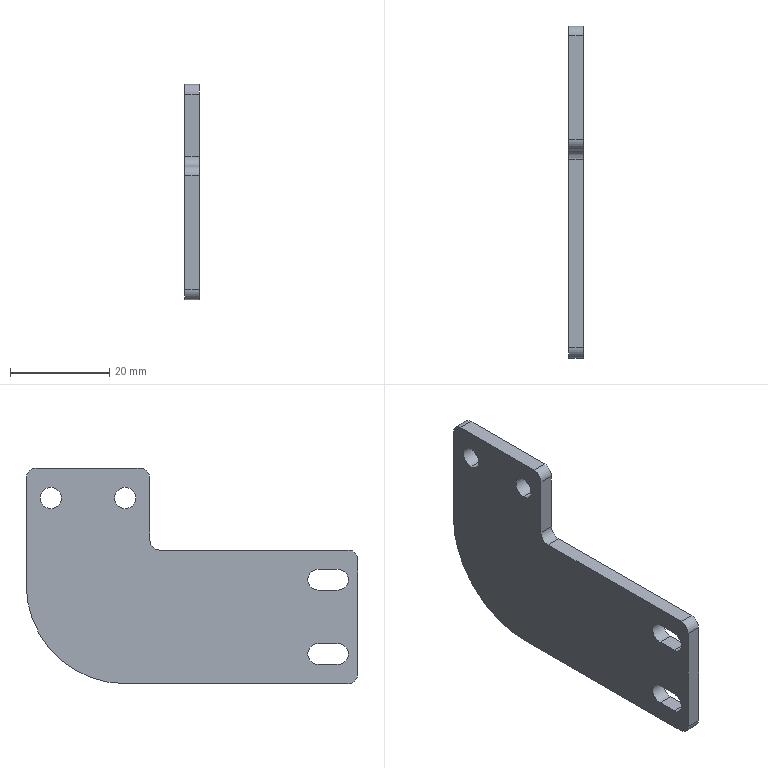Part | SolidWorks | features ICE 5, Fillet 4, Extrusion 1, HoleWzd 1, LPattern 1 | 1 solid | 26 faces | box 3 x 67 x 43.5 mm | volume 6128 mm3 | cylinder 14 | plane 12 | commonest cylinder face diameters 4 x5 4.2 x4 4.3 x4 40 x1
STEP:
#1=CARTESIAN_POINT('',(3.,56.,2.15));
#2=VERTEX_POINT('',#1);
#3=CARTESIAN_POINT('',(3.,56.,-2.15));
#4=VERTEX_POINT('',#3);
#5=CARTESIAN_POINT('',(3.,56.,0.));
#6=DIRECTION('',(1.,0.,0.));
#7=DIRECTION('',(0.,0.,-1.));
#8=AXIS2_PLACEMENT_3D('',#5,#6,#7);
#9=CIRCLE('',#8,2.15);
#10=EDGE_CURVE('',#2,#4,#9,.T.);
#11=ORIENTED_EDGE('',*,*,#10,.T.);
#12=CARTESIAN_POINT('',(0.,56.,-2.15));
#13=VERTEX_POINT('',#12);
#14=CARTESIAN_POINT('',(0.,56.,-2.15));
#15=DIRECTION('',(-1.,0.,0.));
#16=VECTOR('',#15,1000.);
#17=LINE('',#14,#16);
#18=EDGE_CURVE('',#4,#13,#17,.T.);
#19=ORIENTED_EDGE('',*,*,#18,.T.);
#20=CARTESIAN_POINT('',(0.,56.,2.15));
#21=VERTEX_POINT('',#20);
#22=CARTESIAN_POINT('',(0.,56.,0.));
#23=DIRECTION('',(-1.,0.,0.));
#24=DIRECTION('',(0.,0.,1.));
#25=AXIS2_PLACEMENT_3D('',#22,#23,#24);
#26=CIRCLE('',#25,2.15);
#27=EDGE_CURVE('',#13,#21,#26,.T.);
#28=ORIENTED_EDGE('',*,*,#27,.T.);
#29=CARTESIAN_POINT('',(0.,56.,2.15));
#30=DIRECTION('',(-1.,0.,0.));
#31=VECTOR('',#30,1000.);
#32=LINE('',#29,#31);
#33=EDGE_CURVE('',#2,#21,#32,.T.);
#34=ORIENTED_EDGE('',*,*,#33,.F.);
#35=EDGE_LOOP('',(#11,#19,#28,#34));
#36=FACE_OUTER_BOUND('',#35,.T.);
#37=CARTESIAN_POINT('',(0.,56.,0.));
#38=DIRECTION('',(-1.,0.,0.));
#39=DIRECTION('',(0.,0.,1.));
#40=AXIS2_PLACEMENT_3D('',#37,#38,#39);
#41=CYLINDRICAL_SURFACE('',#40,2.15);
#42=ADVANCED_FACE('',(#36),#41,.F.);
#43=CARTESIAN_POINT('',(3.,41.,2.15));
#44=VERTEX_POINT('',#43);
#45=CARTESIAN_POINT('',(3.,41.,-2.15));
#46=VERTEX_POINT('',#45);
#47=CARTESIAN_POINT('',(3.,41.,0.));
#48=DIRECTION('',(1.,0.,0.));
#49=DIRECTION('',(0.,0.,-1.));
#50=AXIS2_PLACEMENT_3D('',#47,#48,#49);
#51=CIRCLE('',#50,2.15);
#52=EDGE_CURVE('',#44,#46,#51,.T.);
#53=ORIENTED_EDGE('',*,*,#52,.T.);
#54=CARTESIAN_POINT('',(0.,41.,-2.15));
#55=VERTEX_POINT('',#54);
#56=CARTESIAN_POINT('',(0.,41.,-2.15));
#57=DIRECTION('',(-1.,0.,0.));
#58=VECTOR('',#57,1000.);
#59=LINE('',#56,#58);
#60=EDGE_CURVE('',#46,#55,#59,.T.);
#61=ORIENTED_EDGE('',*,*,#60,.T.);
#62=CARTESIAN_POINT('',(0.,41.,2.15));
#63=VERTEX_POINT('',#62);
#64=CARTESIAN_POINT('',(0.,41.,0.));
#65=DIRECTION('',(-1.,0.,0.));
#66=DIRECTION('',(0.,0.,1.));
#67=AXIS2_PLACEMENT_3D('',#64,#65,#66);
#68=CIRCLE('',#67,2.15);
#69=EDGE_CURVE('',#55,#63,#68,.T.);
#70=ORIENTED_EDGE('',*,*,#69,.T.);
#71=CARTESIAN_POINT('',(0.,41.,2.15));
#72=DIRECTION('',(-1.,0.,0.));
#73=VECTOR('',#72,1000.);
#74=LINE('',#71,#73);
#75=EDGE_CURVE('',#44,#63,#74,.T.);
#76=ORIENTED_EDGE('',*,*,#75,.F.);
#77=EDGE_LOOP('',(#53,#61,#70,#76));
#78=FACE_OUTER_BOUND('',#77,.T.);
#79=CARTESIAN_POINT('',(0.,41.,0.));
#80=DIRECTION('',(-1.,0.,0.));
#81=DIRECTION('',(0.,0.,1.));
#82=AXIS2_PLACEMENT_3D('',#79,#80,#81);
#83=CYLINDRICAL_SURFACE('',#82,2.15);
#84=ADVANCED_FACE('',(#78),#83,.F.);
#85=CARTESIAN_POINT('',(3.,61.,-17.5));
#86=VERTEX_POINT('',#85);
#87=CARTESIAN_POINT('',(3.,61.,4.));
#88=VERTEX_POINT('',#87);
#89=CARTESIAN_POINT('',(3.,61.,6.));
#90=DIRECTION('',(0.,0.,1.));
#91=VECTOR('',#90,1000.);
#92=LINE('',#89,#91);
#93=EDGE_CURVE('',#86,#88,#92,.T.);
#94=ORIENTED_EDGE('',*,*,#93,.F.);
#95=CARTESIAN_POINT('',(0.,61.,-17.5));
#96=VERTEX_POINT('',#95);
#97=CARTESIAN_POINT('',(0.,61.,-17.5));
#98=DIRECTION('',(-1.,0.,0.));
#99=VECTOR('',#98,1000.);
#100=LINE('',#97,#99);
#101=EDGE_CURVE('',#86,#96,#100,.T.);
#102=ORIENTED_EDGE('',*,*,#101,.T.);
#103=CARTESIAN_POINT('',(0.,61.,4.));
#104=VERTEX_POINT('',#103);
#105=CARTESIAN_POINT('',(0.,61.,6.));
#106=DIRECTION('',(0.,0.,1.));
#107=VECTOR('',#106,1000.);
#108=LINE('',#105,#107);
#109=EDGE_CURVE('',#96,#104,#108,.T.);
#110=ORIENTED_EDGE('',*,*,#109,.T.);
#111=CARTESIAN_POINT('',(3.,61.,4.));
#112=DIRECTION('',(1.,0.,0.));
#113=VECTOR('',#112,1000.);
#114=LINE('',#111,#113);
#115=EDGE_CURVE('',#104,#88,#114,.T.);
#116=ORIENTED_EDGE('',*,*,#115,.T.);
#117=EDGE_LOOP('',(#94,#102,#110,#116));
#118=FACE_OUTER_BOUND('',#117,.T.);
#119=CARTESIAN_POINT('',(3.,61.,6.));
#120=DIRECTION('',(0.,-1.,0.));
#121=DIRECTION('',(0.,0.,-1.));
#122=AXIS2_PLACEMENT_3D('',#119,#120,#121);
#123=PLANE('',#122);
#124=ADVANCED_FACE('',(#118),#123,.F.);
#125=CARTESIAN_POINT('',(3.,-6.,-12.5));
#126=VERTEX_POINT('',#125);
#127=CARTESIAN_POINT('',(3.,-6.,-35.5));
#128=VERTEX_POINT('',#127);
#129=CARTESIAN_POINT('',(3.,-6.,12.5));
#130=DIRECTION('',(0.,0.,-1.));
#131=VECTOR('',#130,1000.);
#132=LINE('',#129,#131);
#133=EDGE_CURVE('',#126,#128,#132,.T.);
#134=ORIENTED_EDGE('',*,*,#133,.F.);
#135=CARTESIAN_POINT('',(0.,-6.,-12.5));
#136=VERTEX_POINT('',#135);
#137=CARTESIAN_POINT('',(0.,-6.,-12.5));
#138=DIRECTION('',(-1.,0.,0.));
#139=VECTOR('',#138,1000.);
#140=LINE('',#137,#139);
#141=EDGE_CURVE('',#126,#136,#140,.T.);
#142=ORIENTED_EDGE('',*,*,#141,.T.);
#143=CARTESIAN_POINT('',(0.,-6.,-35.5));
#144=VERTEX_POINT('',#143);
#145=CARTESIAN_POINT('',(0.,-6.,12.5));
#146=DIRECTION('',(0.,0.,-1.));
#147=VECTOR('',#146,1000.);
#148=LINE('',#145,#147);
#149=EDGE_CURVE('',#136,#144,#148,.T.);
#150=ORIENTED_EDGE('',*,*,#149,.T.);
#151=CARTESIAN_POINT('',(3.,-6.,-35.5));
#152=DIRECTION('',(1.,0.,0.));
#153=VECTOR('',#152,1000.);
#154=LINE('',#151,#153);
#155=EDGE_CURVE('',#144,#128,#154,.T.);
#156=ORIENTED_EDGE('',*,*,#155,.T.);
#157=EDGE_LOOP('',(#134,#142,#150,#156));
#158=FACE_OUTER_BOUND('',#157,.T.);
#159=CARTESIAN_POINT('',(3.,-6.,12.5));
#160=DIRECTION('',(0.,1.,0.));
#161=DIRECTION('',(0.,0.,1.));
#162=AXIS2_PLACEMENT_3D('',#159,#160,#161);
#163=PLANE('',#162);
#164=ADVANCED_FACE('',(#158),#163,.F.);
#165=CARTESIAN_POINT('',(3.,41.,-37.5));
#166=VERTEX_POINT('',#165);
#167=CARTESIAN_POINT('',(3.,-4.,-37.5));
#168=VERTEX_POINT('',#167);
#169=CARTESIAN_POINT('',(3.,61.,-37.5));
#170=DIRECTION('',(0.,-1.,0.));
#171=VECTOR('',#170,1000.);
#172=LINE('',#169,#171);
#173=EDGE_CURVE('',#166,#168,#172,.T.);
#174=ORIENTED_EDGE('',*,*,#173,.F.);
#175=CARTESIAN_POINT('',(3.,41.,-17.5));
#176=DIRECTION('',(1.,0.,0.));
#177=DIRECTION('',(0.,0.,-1.));
#178=AXIS2_PLACEMENT_3D('',#175,#176,#177);
#179=CIRCLE('',#178,20.);
#180=EDGE_CURVE('',#166,#86,#179,.T.);
#181=ORIENTED_EDGE('',*,*,#180,.T.);
#182=ORIENTED_EDGE('',*,*,#93,.T.);
#183=CARTESIAN_POINT('',(3.,59.,6.));
#184=VERTEX_POINT('',#183);
#185=CARTESIAN_POINT('',(3.,59.,4.));
#186=DIRECTION('',(1.,0.,0.));
#187=DIRECTION('',(0.,0.,-1.));
#188=AXIS2_PLACEMENT_3D('',#185,#186,#187);
#189=CIRCLE('',#188,2.);
#190=EDGE_CURVE('',#88,#184,#189,.T.);
#191=ORIENTED_EDGE('',*,*,#190,.T.);
#192=CARTESIAN_POINT('',(3.,38.,6.));
#193=VERTEX_POINT('',#192);
#194=CARTESIAN_POINT('',(3.,0.,6.));
#195=DIRECTION('',(0.,1.,0.));
#196=VECTOR('',#195,1000.);
#197=LINE('',#194,#196);
#198=EDGE_CURVE('',#193,#184,#197,.T.);
#199=ORIENTED_EDGE('',*,*,#198,.F.);
#200=CARTESIAN_POINT('',(3.,36.,4.));
#201=VERTEX_POINT('',#200);
#202=CARTESIAN_POINT('',(3.,38.,4.));
#203=DIRECTION('',(1.,0.,0.));
#204=DIRECTION('',(0.,0.,-1.));
#205=AXIS2_PLACEMENT_3D('',#202,#203,#204);
#206=CIRCLE('',#205,2.);
#207=EDGE_CURVE('',#193,#201,#206,.T.);
#208=ORIENTED_EDGE('',*,*,#207,.T.);
#209=CARTESIAN_POINT('',(3.,36.,-8.5));
#210=VERTEX_POINT('',#209);
#211=CARTESIAN_POINT('',(3.,36.,-3.567));
#212=DIRECTION('',(0.,0.,1.));
#213=VECTOR('',#212,1000.);
#214=LINE('',#211,#213);
#215=EDGE_CURVE('',#210,#201,#214,.T.);
#216=ORIENTED_EDGE('',*,*,#215,.F.);
#217=CARTESIAN_POINT('',(3.,34.,-10.5));
#218=VERTEX_POINT('',#217);
#219=CARTESIAN_POINT('',(3.,34.,-8.5));
#220=DIRECTION('',(-1.,0.,0.));
#221=DIRECTION('',(0.,0.,-1.));
#222=AXIS2_PLACEMENT_3D('',#219,#220,#221);
#223=CIRCLE('',#222,2.);
#224=EDGE_CURVE('',#210,#218,#223,.T.);
#225=ORIENTED_EDGE('',*,*,#224,.T.);
#226=CARTESIAN_POINT('',(3.,-4.,-10.5));
#227=VERTEX_POINT('',#226);
#228=CARTESIAN_POINT('',(3.,-6.,-10.5));
#229=DIRECTION('',(0.,1.,0.));
#230=VECTOR('',#229,1000.);
#231=LINE('',#228,#230);
#232=EDGE_CURVE('',#227,#218,#231,.T.);
#233=ORIENTED_EDGE('',*,*,#232,.F.);
#234=CARTESIAN_POINT('',(3.,-4.,-12.5));
#235=DIRECTION('',(1.,0.,0.));
#236=DIRECTION('',(0.,0.,-1.));
#237=AXIS2_PLACEMENT_3D('',#234,#235,#236);
#238=CIRCLE('',#237,2.);
#239=EDGE_CURVE('',#227,#126,#238,.T.);
#240=ORIENTED_EDGE('',*,*,#239,.T.);
#241=ORIENTED_EDGE('',*,*,#133,.T.);
#242=CARTESIAN_POINT('',(3.,-4.,-35.5));
#243=DIRECTION('',(1.,0.,0.));
#244=DIRECTION('',(0.,0.,-1.));
#245=AXIS2_PLACEMENT_3D('',#242,#243,#244);
#246=CIRCLE('',#245,2.);
#247=EDGE_CURVE('',#128,#168,#246,.T.);
#248=ORIENTED_EDGE('',*,*,#247,.T.);
#249=EDGE_LOOP('',(#174,#181,#182,#191,#199,#208,#216,#225,#233,#240,#241,#248));
#250=FACE_OUTER_BOUND('',#249,.T.);
#251=CARTESIAN_POINT('',(3.,2.,-14.4));
#252=VERTEX_POINT('',#251);
#253=CARTESIAN_POINT('',(3.,2.,-18.6));
#254=VERTEX_POINT('',#253);
#255=CARTESIAN_POINT('',(3.,2.,-16.5));
#256=DIRECTION('',(-1.,0.,0.));
#257=DIRECTION('',(0.,0.,-1.));
#258=AXIS2_PLACEMENT_3D('',#255,#256,#257);
#259=CIRCLE('',#258,2.1);
#260=EDGE_CURVE('',#252,#254,#259,.T.);
#261=ORIENTED_EDGE('',*,*,#260,.T.);
#262=CARTESIAN_POINT('',(3.,-2.,-18.6));
#263=VERTEX_POINT('',#262);
#264=CARTESIAN_POINT('',(3.,2.,-18.6));
#265=DIRECTION('',(0.,-1.,0.));
#266=VECTOR('',#265,1000.);
#267=LINE('',#264,#266);
#268=EDGE_CURVE('',#254,#263,#267,.T.);
#269=ORIENTED_EDGE('',*,*,#268,.T.);
#270=CARTESIAN_POINT('',(3.,-2.,-14.4));
#271=VERTEX_POINT('',#270);
#272=CARTESIAN_POINT('',(3.,-2.,-16.5));
#273=DIRECTION('',(-1.,0.,0.));
#274=DIRECTION('',(0.,0.,-1.));
#275=AXIS2_PLACEMENT_3D('',#272,#273,#274);
#276=CIRCLE('',#275,2.1);
#277=EDGE_CURVE('',#263,#271,#276,.T.);
#278=ORIENTED_EDGE('',*,*,#277,.T.);
#279=CARTESIAN_POINT('',(3.,2.,-14.4));
#280=DIRECTION('',(0.,1.,0.));
#281=VECTOR('',#280,1000.);
#282=LINE('',#279,#281);
#283=EDGE_CURVE('',#271,#252,#282,.T.);
#284=ORIENTED_EDGE('',*,*,#283,.T.);
#285=EDGE_LOOP('',(#261,#269,#278,#284));
#286=FACE_BOUND('',#285,.T.);
#287=CARTESIAN_POINT('',(3.,2.,-29.4));
#288=VERTEX_POINT('',#287);
#289=CARTESIAN_POINT('',(3.,2.,-33.6));
#290=VERTEX_POINT('',#289);
#291=CARTESIAN_POINT('',(3.,2.,-31.5));
#292=DIRECTION('',(-1.,0.,0.));
#293=DIRECTION('',(0.,0.,1.));
#294=AXIS2_PLACEMENT_3D('',#291,#292,#293);
#295=CIRCLE('',#294,2.1);
#296=EDGE_CURVE('',#288,#290,#295,.T.);
#297=ORIENTED_EDGE('',*,*,#296,.T.);
#298=CARTESIAN_POINT('',(3.,-2.,-33.6));
#299=VERTEX_POINT('',#298);
#300=CARTESIAN_POINT('',(3.,2.,-33.6));
#301=DIRECTION('',(0.,-1.,0.));
#302=VECTOR('',#301,1000.);
#303=LINE('',#300,#302);
#304=EDGE_CURVE('',#290,#299,#303,.T.);
#305=ORIENTED_EDGE('',*,*,#304,.T.);
#306=CARTESIAN_POINT('',(3.,-2.,-29.4));
#307=VERTEX_POINT('',#306);
#308=CARTESIAN_POINT('',(3.,-2.,-31.5));
#309=DIRECTION('',(-1.,0.,0.));
#310=DIRECTION('',(0.,0.,1.));
#311=AXIS2_PLACEMENT_3D('',#308,#309,#310);
#312=CIRCLE('',#311,2.1);
#313=EDGE_CURVE('',#299,#307,#312,.T.);
#314=ORIENTED_EDGE('',*,*,#313,.T.);
#315=CARTESIAN_POINT('',(3.,2.,-29.4));
#316=DIRECTION('',(0.,1.,0.));
#317=VECTOR('',#316,1000.);
#318=LINE('',#315,#317);
#319=EDGE_CURVE('',#307,#288,#318,.T.);
#320=ORIENTED_EDGE('',*,*,#319,.T.);
#321=EDGE_LOOP('',(#297,#305,#314,#320));
#322=FACE_BOUND('',#321,.T.);
#323=ORIENTED_EDGE('',*,*,#10,.F.);
#324=CARTESIAN_POINT('',(3.,56.,0.));
#325=DIRECTION('',(1.,0.,0.));
#326=DIRECTION('',(0.,0.,-1.));
#327=AXIS2_PLACEMENT_3D('',#324,#325,#326);
#328=CIRCLE('',#327,2.15);
#329=EDGE_CURVE('',#4,#2,#328,.T.);
#330=ORIENTED_EDGE('',*,*,#329,.F.);
#331=EDGE_LOOP('',(#323,#330));
#332=FACE_BOUND('',#331,.T.);
#333=ORIENTED_EDGE('',*,*,#52,.F.);
#334=CARTESIAN_POINT('',(3.,41.,0.));
#335=DIRECTION('',(1.,0.,0.));
#336=DIRECTION('',(0.,0.,-1.));
#337=AXIS2_PLACEMENT_3D('',#334,#335,#336);
#338=CIRCLE('',#337,2.15);
#339=EDGE_CURVE('',#46,#44,#338,.T.);
#340=ORIENTED_EDGE('',*,*,#339,.F.);
#341=EDGE_LOOP('',(#333,#340));
#342=FACE_BOUND('',#341,.T.);
#343=CARTESIAN_POINT('',(3.,0.,0.));
#344=DIRECTION('',(1.,0.,0.));
#345=DIRECTION('',(0.,0.,-1.));
#346=AXIS2_PLACEMENT_3D('',#343,#344,#345);
#347=PLANE('',#346);
#348=ADVANCED_FACE('',(#250,#286,#322,#332,#342),#347,.T.);
#349=CARTESIAN_POINT('',(0.,2.,-18.6));
#350=VERTEX_POINT('',#349);
#351=CARTESIAN_POINT('',(0.,-2.,-18.6));
#352=VERTEX_POINT('',#351);
#353=CARTESIAN_POINT('',(0.,2.,-18.6));
#354=DIRECTION('',(0.,-1.,0.));
#355=VECTOR('',#354,1000.);
#356=LINE('',#353,#355);
#357=EDGE_CURVE('',#350,#352,#356,.T.);
#358=ORIENTED_EDGE('',*,*,#357,.F.);
#359=CARTESIAN_POINT('',(0.,2.,-14.4));
#360=VERTEX_POINT('',#359);
#361=CARTESIAN_POINT('',(0.,2.,-16.5));
#362=DIRECTION('',(-1.,0.,0.));
#363=DIRECTION('',(0.,0.,-1.));
#364=AXIS2_PLACEMENT_3D('',#361,#362,#363);
#365=CIRCLE('',#364,2.1);
#366=EDGE_CURVE('',#360,#350,#365,.T.);
#367=ORIENTED_EDGE('',*,*,#366,.F.);
#368=CARTESIAN_POINT('',(0.,-2.,-14.4));
#369=VERTEX_POINT('',#368);
#370=CARTESIAN_POINT('',(0.,2.,-14.4));
#371=DIRECTION('',(0.,1.,0.));
#372=VECTOR('',#371,1000.);
#373=LINE('',#370,#372);
#374=EDGE_CURVE('',#369,#360,#373,.T.);
#375=ORIENTED_EDGE('',*,*,#374,.F.);
#376=CARTESIAN_POINT('',(0.,-2.,-16.5));
#377=DIRECTION('',(-1.,0.,0.));
#378=DIRECTION('',(0.,0.,-1.));
#379=AXIS2_PLACEMENT_3D('',#376,#377,#378);
#380=CIRCLE('',#379,2.1);
#381=EDGE_CURVE('',#352,#369,#380,.T.);
#382=ORIENTED_EDGE('',*,*,#381,.F.);
#383=EDGE_LOOP('',(#358,#367,#375,#382));
#384=FACE_BOUND('',#383,.T.);
#385=CARTESIAN_POINT('',(0.,2.,-33.6));
#386=VERTEX_POINT('',#385);
#387=CARTESIAN_POINT('',(0.,-2.,-33.6));
#388=VERTEX_POINT('',#387);
#389=CARTESIAN_POINT('',(0.,2.,-33.6));
#390=DIRECTION('',(0.,-1.,0.));
#391=VECTOR('',#390,1000.);
#392=LINE('',#389,#391);
#393=EDGE_CURVE('',#386,#388,#392,.T.);
#394=ORIENTED_EDGE('',*,*,#393,.F.);
#395=CARTESIAN_POINT('',(0.,2.,-29.4));
#396=VERTEX_POINT('',#395);
#397=CARTESIAN_POINT('',(0.,2.,-31.5));
#398=DIRECTION('',(-1.,0.,0.));
#399=DIRECTION('',(0.,0.,1.));
#400=AXIS2_PLACEMENT_3D('',#397,#398,#399);
#401=CIRCLE('',#400,2.1);
#402=EDGE_CURVE('',#396,#386,#401,.T.);
#403=ORIENTED_EDGE('',*,*,#402,.F.);
#404=CARTESIAN_POINT('',(0.,-2.,-29.4));
#405=VERTEX_POINT('',#404);
#406=CARTESIAN_POINT('',(0.,2.,-29.4));
#407=DIRECTION('',(0.,1.,0.));
#408=VECTOR('',#407,1000.);
#409=LINE('',#406,#408);
#410=EDGE_CURVE('',#405,#396,#409,.T.);
#411=ORIENTED_EDGE('',*,*,#410,.F.);
#412=CARTESIAN_POINT('',(0.,-2.,-31.5));
#413=DIRECTION('',(-1.,0.,0.));
#414=DIRECTION('',(0.,0.,1.));
#415=AXIS2_PLACEMENT_3D('',#412,#413,#414);
#416=CIRCLE('',#415,2.1);
#417=EDGE_CURVE('',#388,#405,#416,.T.);
#418=ORIENTED_EDGE('',*,*,#417,.F.);
#419=EDGE_LOOP('',(#394,#403,#411,#418));
#420=FACE_BOUND('',#419,.T.);
#421=ORIENTED_EDGE('',*,*,#109,.F.);
#422=CARTESIAN_POINT('',(0.,41.,-37.5));
#423=VERTEX_POINT('',#422);
#424=CARTESIAN_POINT('',(0.,41.,-17.5));
#425=DIRECTION('',(-1.,0.,0.));
#426=DIRECTION('',(0.,0.,-1.));
#427=AXIS2_PLACEMENT_3D('',#424,#425,#426);
#428=CIRCLE('',#427,20.);
#429=EDGE_CURVE('',#96,#423,#428,.T.);
#430=ORIENTED_EDGE('',*,*,#429,.T.);
#431=CARTESIAN_POINT('',(0.,-4.,-37.5));
#432=VERTEX_POINT('',#431);
#433=CARTESIAN_POINT('',(0.,61.,-37.5));
#434=DIRECTION('',(0.,-1.,0.));
#435=VECTOR('',#434,1000.);
#436=LINE('',#433,#435);
#437=EDGE_CURVE('',#423,#432,#436,.T.);
#438=ORIENTED_EDGE('',*,*,#437,.T.);
#439=CARTESIAN_POINT('',(0.,-4.,-35.5));
#440=DIRECTION('',(-1.,0.,0.));
#441=DIRECTION('',(0.,0.,-1.));
#442=AXIS2_PLACEMENT_3D('',#439,#440,#441);
#443=CIRCLE('',#442,2.);
#444=EDGE_CURVE('',#432,#144,#443,.T.);
#445=ORIENTED_EDGE('',*,*,#444,.T.);
#446=ORIENTED_EDGE('',*,*,#149,.F.);
#447=CARTESIAN_POINT('',(0.,-4.,-10.5));
#448=VERTEX_POINT('',#447);
#449=CARTESIAN_POINT('',(0.,-4.,-12.5));
#450=DIRECTION('',(-1.,0.,0.));
#451=DIRECTION('',(0.,0.,-1.));
#452=AXIS2_PLACEMENT_3D('',#449,#450,#451);
#453=CIRCLE('',#452,2.);
#454=EDGE_CURVE('',#136,#448,#453,.T.);
#455=ORIENTED_EDGE('',*,*,#454,.T.);
#456=CARTESIAN_POINT('',(0.,34.,-10.5));
#457=VERTEX_POINT('',#456);
#458=CARTESIAN_POINT('',(0.,-6.,-10.5));
#459=DIRECTION('',(0.,1.,0.));
#460=VECTOR('',#459,1000.);
#461=LINE('',#458,#460);
#462=EDGE_CURVE('',#448,#457,#461,.T.);
#463=ORIENTED_EDGE('',*,*,#462,.T.);
#464=CARTESIAN_POINT('',(0.,36.,-8.5));
#465=VERTEX_POINT('',#464);
#466=CARTESIAN_POINT('',(0.,34.,-8.5));
#467=DIRECTION('',(1.,0.,0.));
#468=DIRECTION('',(0.,0.,-1.));
#469=AXIS2_PLACEMENT_3D('',#466,#467,#468);
#470=CIRCLE('',#469,2.);
#471=EDGE_CURVE('',#457,#465,#470,.T.);
#472=ORIENTED_EDGE('',*,*,#471,.T.);
#473=CARTESIAN_POINT('',(0.,36.,4.));
#474=VERTEX_POINT('',#473);
#475=CARTESIAN_POINT('',(0.,36.,-3.567));
#476=DIRECTION('',(0.,0.,1.));
#477=VECTOR('',#476,1000.);
#478=LINE('',#475,#477);
#479=EDGE_CURVE('',#465,#474,#478,.T.);
#480=ORIENTED_EDGE('',*,*,#479,.T.);
#481=CARTESIAN_POINT('',(0.,38.,6.));
#482=VERTEX_POINT('',#481);
#483=CARTESIAN_POINT('',(0.,38.,4.));
#484=DIRECTION('',(-1.,0.,0.));
#485=DIRECTION('',(0.,0.,-1.));
#486=AXIS2_PLACEMENT_3D('',#483,#484,#485);
#487=CIRCLE('',#486,2.);
#488=EDGE_CURVE('',#474,#482,#487,.T.);
#489=ORIENTED_EDGE('',*,*,#488,.T.);
#490=CARTESIAN_POINT('',(0.,59.,6.));
#491=VERTEX_POINT('',#490);
#492=CARTESIAN_POINT('',(0.,61.,6.));
#493=DIRECTION('',(0.,-1.,0.));
#494=VECTOR('',#493,1000.);
#495=LINE('',#492,#494);
#496=EDGE_CURVE('',#491,#482,#495,.T.);
#497=ORIENTED_EDGE('',*,*,#496,.F.);
#498=CARTESIAN_POINT('',(0.,59.,4.));
#499=DIRECTION('',(-1.,0.,0.));
#500=DIRECTION('',(0.,0.,-1.));
#501=AXIS2_PLACEMENT_3D('',#498,#499,#500);
#502=CIRCLE('',#501,2.);
#503=EDGE_CURVE('',#491,#104,#502,.T.);
#504=ORIENTED_EDGE('',*,*,#503,.T.);
#505=EDGE_LOOP('',(#421,#430,#438,#445,#446,#455,#463,#472,#480,#489,#497,#504));
#506=FACE_OUTER_BOUND('',#505,.T.);
#507=CARTESIAN_POINT('',(0.,56.,0.));
#508=DIRECTION('',(-1.,0.,0.));
#509=DIRECTION('',(0.,0.,1.));
#510=AXIS2_PLACEMENT_3D('',#507,#508,#509);
#511=CIRCLE('',#510,2.15);
#512=EDGE_CURVE('',#21,#13,#511,.T.);
#513=ORIENTED_EDGE('',*,*,#512,.F.);
#514=ORIENTED_EDGE('',*,*,#27,.F.);
#515=EDGE_LOOP('',(#513,#514));
#516=FACE_BOUND('',#515,.T.);
#517=CARTESIAN_POINT('',(0.,41.,0.));
#518=DIRECTION('',(-1.,0.,0.));
#519=DIRECTION('',(0.,0.,1.));
#520=AXIS2_PLACEMENT_3D('',#517,#518,#519);
#521=CIRCLE('',#520,2.15);
#522=EDGE_CURVE('',#63,#55,#521,.T.);
#523=ORIENTED_EDGE('',*,*,#522,.F.);
#524=ORIENTED_EDGE('',*,*,#69,.F.);
#525=EDGE_LOOP('',(#523,#524));
#526=FACE_BOUND('',#525,.T.);
#527=CARTESIAN_POINT('',(0.,0.,0.));
#528=DIRECTION('',(1.,0.,0.));
#529=DIRECTION('',(0.,0.,-1.));
#530=AXIS2_PLACEMENT_3D('',#527,#528,#529);
#531=PLANE('',#530);
#532=ADVANCED_FACE('',(#384,#420,#506,#516,#526),#531,.F.);
#533=ORIENTED_EDGE('',*,*,#60,.F.);
#534=ORIENTED_EDGE('',*,*,#339,.T.);
#535=ORIENTED_EDGE('',*,*,#75,.T.);
#536=ORIENTED_EDGE('',*,*,#522,.T.);
#537=EDGE_LOOP('',(#533,#534,#535,#536));
#538=FACE_OUTER_BOUND('',#537,.T.);
#539=CARTESIAN_POINT('',(0.,41.,0.));
#540=DIRECTION('',(-1.,0.,0.));
#541=DIRECTION('',(0.,0.,1.));
#542=AXIS2_PLACEMENT_3D('',#539,#540,#541);
#543=CYLINDRICAL_SURFACE('',#542,2.15);
#544=ADVANCED_FACE('',(#538),#543,.F.);
#545=ORIENTED_EDGE('',*,*,#18,.F.);
#546=ORIENTED_EDGE('',*,*,#329,.T.);
#547=ORIENTED_EDGE('',*,*,#33,.T.);
#548=ORIENTED_EDGE('',*,*,#512,.T.);
#549=EDGE_LOOP('',(#545,#546,#547,#548));
#550=FACE_OUTER_BOUND('',#549,.T.);
#551=CARTESIAN_POINT('',(0.,56.,0.));
#552=DIRECTION('',(-1.,0.,0.));
#553=DIRECTION('',(0.,0.,1.));
#554=AXIS2_PLACEMENT_3D('',#551,#552,#553);
#555=CYLINDRICAL_SURFACE('',#554,2.15);
#556=ADVANCED_FACE('',(#550),#555,.F.);
#557=ORIENTED_EDGE('',*,*,#437,.F.);
#558=CARTESIAN_POINT('',(3.,41.,-37.5));
#559=DIRECTION('',(1.,0.,0.));
#560=VECTOR('',#559,1000.);
#561=LINE('',#558,#560);
#562=EDGE_CURVE('',#423,#166,#561,.T.);
#563=ORIENTED_EDGE('',*,*,#562,.T.);
#564=ORIENTED_EDGE('',*,*,#173,.T.);
#565=CARTESIAN_POINT('',(0.,-4.,-37.5));
#566=DIRECTION('',(-1.,0.,0.));
#567=VECTOR('',#566,1000.);
#568=LINE('',#565,#567);
#569=EDGE_CURVE('',#168,#432,#568,.T.);
#570=ORIENTED_EDGE('',*,*,#569,.T.);
#571=EDGE_LOOP('',(#557,#563,#564,#570));
#572=FACE_OUTER_BOUND('',#571,.T.);
#573=CARTESIAN_POINT('',(78.103,61.,-37.5));
#574=DIRECTION('',(0.,0.,-1.));
#575=DIRECTION('',(0.,1.,0.));
#576=AXIS2_PLACEMENT_3D('',#573,#574,#575);
#577=PLANE('',#576);
#578=ADVANCED_FACE('',(#572),#577,.T.);
#579=ORIENTED_EDGE('',*,*,#462,.F.);
#580=CARTESIAN_POINT('',(3.,-4.,-10.5));
#581=DIRECTION('',(1.,0.,0.));
#582=VECTOR('',#581,1000.);
#583=LINE('',#580,#582);
#584=EDGE_CURVE('',#448,#227,#583,.T.);
#585=ORIENTED_EDGE('',*,*,#584,.T.);
#586=ORIENTED_EDGE('',*,*,#232,.T.);
#587=CARTESIAN_POINT('',(0.,34.,-10.5));
#588=DIRECTION('',(-1.,0.,0.));
#589=VECTOR('',#588,1000.);
#590=LINE('',#587,#589);
#591=EDGE_CURVE('',#218,#457,#590,.T.);
#592=ORIENTED_EDGE('',*,*,#591,.T.);
#593=EDGE_LOOP('',(#579,#585,#586,#592));
#594=FACE_OUTER_BOUND('',#593,.T.);
#595=CARTESIAN_POINT('',(78.103,-6.,-10.5));
#596=DIRECTION('',(0.,0.,1.));
#597=DIRECTION('',(1.,0.,0.));
#598=AXIS2_PLACEMENT_3D('',#595,#596,#597);
#599=PLANE('',#598);
#600=ADVANCED_FACE('',(#594),#599,.T.);
#601=ORIENTED_EDGE('',*,*,#479,.F.);
#602=CARTESIAN_POINT('',(3.,36.,-8.5));
#603=DIRECTION('',(1.,0.,0.));
#604=VECTOR('',#603,1000.);
#605=LINE('',#602,#604);
#606=EDGE_CURVE('',#465,#210,#605,.T.);
#607=ORIENTED_EDGE('',*,*,#606,.T.);
#608=ORIENTED_EDGE('',*,*,#215,.T.);
#609=CARTESIAN_POINT('',(0.,36.,4.));
#610=DIRECTION('',(-1.,0.,0.));
#611=VECTOR('',#610,1000.);
#612=LINE('',#609,#611);
#613=EDGE_CURVE('',#201,#474,#612,.T.);
#614=ORIENTED_EDGE('',*,*,#613,.T.);
#615=EDGE_LOOP('',(#601,#607,#608,#614));
#616=FACE_OUTER_BOUND('',#615,.T.);
#617=CARTESIAN_POINT('',(78.103,36.,-3.567));
#618=DIRECTION('',(0.,-1.,0.));
#619=DIRECTION('',(0.,0.,-1.));
#620=AXIS2_PLACEMENT_3D('',#617,#618,#619);
#621=PLANE('',#620);
#622=ADVANCED_FACE('',(#616),#621,.T.);
#623=ORIENTED_EDGE('',*,*,#402,.T.);
#624=CARTESIAN_POINT('',(3.,2.,-33.6));
#625=DIRECTION('',(-1.,0.,0.));
#626=VECTOR('',#625,1000.);
#627=LINE('',#624,#626);
#628=EDGE_CURVE('',#290,#386,#627,.T.);
#629=ORIENTED_EDGE('',*,*,#628,.F.);
#630=ORIENTED_EDGE('',*,*,#296,.F.);
#631=CARTESIAN_POINT('',(3.,2.,-29.4));
#632=DIRECTION('',(-1.,0.,0.));
#633=VECTOR('',#632,1000.);
#634=LINE('',#631,#633);
#635=EDGE_CURVE('',#288,#396,#634,.T.);
#636=ORIENTED_EDGE('',*,*,#635,.T.);
#637=EDGE_LOOP('',(#623,#629,#630,#636));
#638=FACE_OUTER_BOUND('',#637,.T.);
#639=CARTESIAN_POINT('',(3.,2.,-31.5));
#640=DIRECTION('',(-1.,0.,0.));
#641=DIRECTION('',(0.,0.,1.));
#642=AXIS2_PLACEMENT_3D('',#639,#640,#641);
#643=CYLINDRICAL_SURFACE('',#642,2.1);
#644=ADVANCED_FACE('',(#638),#643,.F.);
#645=ORIENTED_EDGE('',*,*,#410,.T.);
#646=ORIENTED_EDGE('',*,*,#635,.F.);
#647=ORIENTED_EDGE('',*,*,#319,.F.);
#648=CARTESIAN_POINT('',(3.,-2.,-29.4));
#649=DIRECTION('',(-1.,0.,0.));
#650=VECTOR('',#649,1000.);
#651=LINE('',#648,#650);
#652=EDGE_CURVE('',#307,#405,#651,.T.);
#653=ORIENTED_EDGE('',*,*,#652,.T.);
#654=EDGE_LOOP('',(#645,#646,#647,#653));
#655=FACE_OUTER_BOUND('',#654,.T.);
#656=CARTESIAN_POINT('',(3.,2.,-29.4));
#657=DIRECTION('',(0.,0.,1.));
#658=DIRECTION('',(1.,0.,0.));
#659=AXIS2_PLACEMENT_3D('',#656,#657,#658);
#660=PLANE('',#659);
#661=ADVANCED_FACE('',(#655),#660,.F.);
#662=ORIENTED_EDGE('',*,*,#417,.T.);
#663=ORIENTED_EDGE('',*,*,#652,.F.);
#664=ORIENTED_EDGE('',*,*,#313,.F.);
#665=CARTESIAN_POINT('',(3.,-2.,-33.6));
#666=DIRECTION('',(-1.,0.,0.));
#667=VECTOR('',#666,1000.);
#668=LINE('',#665,#667);
#669=EDGE_CURVE('',#299,#388,#668,.T.);
#670=ORIENTED_EDGE('',*,*,#669,.T.);
#671=EDGE_LOOP('',(#662,#663,#664,#670));
#672=FACE_OUTER_BOUND('',#671,.T.);
#673=CARTESIAN_POINT('',(3.,-2.,-31.5));
#674=DIRECTION('',(-1.,0.,0.));
#675=DIRECTION('',(0.,0.,1.));
#676=AXIS2_PLACEMENT_3D('',#673,#674,#675);
#677=CYLINDRICAL_SURFACE('',#676,2.1);
#678=ADVANCED_FACE('',(#672),#677,.F.);
#679=ORIENTED_EDGE('',*,*,#393,.T.);
#680=ORIENTED_EDGE('',*,*,#669,.F.);
#681=ORIENTED_EDGE('',*,*,#304,.F.);
#682=ORIENTED_EDGE('',*,*,#628,.T.);
#683=EDGE_LOOP('',(#679,#680,#681,#682));
#684=FACE_OUTER_BOUND('',#683,.T.);
#685=CARTESIAN_POINT('',(3.,2.,-33.6));
#686=DIRECTION('',(0.,0.,-1.));
#687=DIRECTION('',(-1.,0.,0.));
#688=AXIS2_PLACEMENT_3D('',#685,#686,#687);
#689=PLANE('',#688);
#690=ADVANCED_FACE('',(#684),#689,.F.);
#691=ORIENTED_EDGE('',*,*,#366,.T.);
#692=CARTESIAN_POINT('',(3.,2.,-18.6));
#693=DIRECTION('',(-1.,0.,0.));
#694=VECTOR('',#693,1000.);
#695=LINE('',#692,#694);
#696=EDGE_CURVE('',#254,#350,#695,.T.);
#697=ORIENTED_EDGE('',*,*,#696,.F.);
#698=ORIENTED_EDGE('',*,*,#260,.F.);
#699=CARTESIAN_POINT('',(3.,2.,-14.4));
#700=DIRECTION('',(-1.,0.,0.));
#701=VECTOR('',#700,1000.);
#702=LINE('',#699,#701);
#703=EDGE_CURVE('',#252,#360,#702,.T.);
#704=ORIENTED_EDGE('',*,*,#703,.T.);
#705=EDGE_LOOP('',(#691,#697,#698,#704));
#706=FACE_OUTER_BOUND('',#705,.T.);
#707=CARTESIAN_POINT('',(3.,2.,-16.5));
#708=DIRECTION('',(-1.,0.,0.));
#709=DIRECTION('',(0.,0.,1.));
#710=AXIS2_PLACEMENT_3D('',#707,#708,#709);
#711=CYLINDRICAL_SURFACE('',#710,2.1);
#712=ADVANCED_FACE('',(#706),#711,.F.);
#713=ORIENTED_EDGE('',*,*,#374,.T.);
#714=ORIENTED_EDGE('',*,*,#703,.F.);
#715=ORIENTED_EDGE('',*,*,#283,.F.);
#716=CARTESIAN_POINT('',(3.,-2.,-14.4));
#717=DIRECTION('',(-1.,0.,0.));
#718=VECTOR('',#717,1000.);
#719=LINE('',#716,#718);
#720=EDGE_CURVE('',#271,#369,#719,.T.);
#721=ORIENTED_EDGE('',*,*,#720,.T.);
#722=EDGE_LOOP('',(#713,#714,#715,#721));
#723=FACE_OUTER_BOUND('',#722,.T.);
#724=CARTESIAN_POINT('',(3.,2.,-14.4));
#725=DIRECTION('',(0.,0.,1.));
#726=DIRECTION('',(1.,0.,0.));
#727=AXIS2_PLACEMENT_3D('',#724,#725,#726);
#728=PLANE('',#727);
#729=ADVANCED_FACE('',(#723),#728,.F.);
#730=ORIENTED_EDGE('',*,*,#381,.T.);
#731=ORIENTED_EDGE('',*,*,#720,.F.);
#732=ORIENTED_EDGE('',*,*,#277,.F.);
#733=CARTESIAN_POINT('',(3.,-2.,-18.6));
#734=DIRECTION('',(-1.,0.,0.));
#735=VECTOR('',#734,1000.);
#736=LINE('',#733,#735);
#737=EDGE_CURVE('',#263,#352,#736,.T.);
#738=ORIENTED_EDGE('',*,*,#737,.T.);
#739=EDGE_LOOP('',(#730,#731,#732,#738));
#740=FACE_OUTER_BOUND('',#739,.T.);
#741=CARTESIAN_POINT('',(3.,-2.,-16.5));
#742=DIRECTION('',(-1.,0.,0.));
#743=DIRECTION('',(0.,0.,1.));
#744=AXIS2_PLACEMENT_3D('',#741,#742,#743);
#745=CYLINDRICAL_SURFACE('',#744,2.1);
#746=ADVANCED_FACE('',(#740),#745,.F.);
#747=ORIENTED_EDGE('',*,*,#357,.T.);
#748=ORIENTED_EDGE('',*,*,#737,.F.);
#749=ORIENTED_EDGE('',*,*,#268,.F.);
#750=ORIENTED_EDGE('',*,*,#696,.T.);
#751=EDGE_LOOP('',(#747,#748,#749,#750));
#752=FACE_OUTER_BOUND('',#751,.T.);
#753=CARTESIAN_POINT('',(3.,2.,-18.6));
#754=DIRECTION('',(0.,0.,-1.));
#755=DIRECTION('',(-1.,0.,0.));
#756=AXIS2_PLACEMENT_3D('',#753,#754,#755);
#757=PLANE('',#756);
#758=ADVANCED_FACE('',(#752),#757,.F.);
#759=ORIENTED_EDGE('',*,*,#496,.T.);
#760=CARTESIAN_POINT('',(3.,38.,6.));
#761=DIRECTION('',(1.,0.,0.));
#762=VECTOR('',#761,1000.);
#763=LINE('',#760,#762);
#764=EDGE_CURVE('',#482,#193,#763,.T.);
#765=ORIENTED_EDGE('',*,*,#764,.T.);
#766=ORIENTED_EDGE('',*,*,#198,.T.);
#767=CARTESIAN_POINT('',(10.,59.,6.));
#768=DIRECTION('',(-1.,0.,0.));
#769=VECTOR('',#768,1000.);
#770=LINE('',#767,#769);
#771=EDGE_CURVE('',#184,#491,#770,.T.);
#772=ORIENTED_EDGE('',*,*,#771,.T.);
#773=EDGE_LOOP('',(#759,#765,#766,#772));
#774=FACE_OUTER_BOUND('',#773,.T.);
#775=CARTESIAN_POINT('',(10.,61.,6.));
#776=DIRECTION('',(0.,0.,-1.));
#777=DIRECTION('',(-1.,0.,0.));
#778=AXIS2_PLACEMENT_3D('',#775,#776,#777);
#779=PLANE('',#778);
#780=ADVANCED_FACE('',(#774),#779,.F.);
#781=ORIENTED_EDGE('',*,*,#239,.F.);
#782=ORIENTED_EDGE('',*,*,#584,.F.);
#783=ORIENTED_EDGE('',*,*,#454,.F.);
#784=ORIENTED_EDGE('',*,*,#141,.F.);
#785=EDGE_LOOP('',(#781,#782,#783,#784));
#786=FACE_OUTER_BOUND('',#785,.T.);
#787=CARTESIAN_POINT('',(3.,-4.,-12.5));
#788=DIRECTION('',(1.,0.,0.));
#789=DIRECTION('',(0.,0.,-1.));
#790=AXIS2_PLACEMENT_3D('',#787,#788,#789);
#791=CYLINDRICAL_SURFACE('',#790,2.);
#792=ADVANCED_FACE('',(#786),#791,.T.);
#793=ORIENTED_EDGE('',*,*,#247,.F.);
#794=ORIENTED_EDGE('',*,*,#155,.F.);
#795=ORIENTED_EDGE('',*,*,#444,.F.);
#796=ORIENTED_EDGE('',*,*,#569,.F.);
#797=EDGE_LOOP('',(#793,#794,#795,#796));
#798=FACE_OUTER_BOUND('',#797,.T.);
#799=CARTESIAN_POINT('',(78.103,-4.,-35.5));
#800=DIRECTION('',(1.,0.,0.));
#801=DIRECTION('',(0.,0.,-1.));
#802=AXIS2_PLACEMENT_3D('',#799,#800,#801);
#803=CYLINDRICAL_SURFACE('',#802,2.);
#804=ADVANCED_FACE('',(#798),#803,.T.);
#805=ORIENTED_EDGE('',*,*,#224,.F.);
#806=ORIENTED_EDGE('',*,*,#606,.F.);
#807=ORIENTED_EDGE('',*,*,#471,.F.);
#808=ORIENTED_EDGE('',*,*,#591,.F.);
#809=EDGE_LOOP('',(#805,#806,#807,#808));
#810=FACE_OUTER_BOUND('',#809,.T.);
#811=CARTESIAN_POINT('',(78.103,34.,-8.5));
#812=DIRECTION('',(1.,0.,0.));
#813=DIRECTION('',(0.,0.,-1.));
#814=AXIS2_PLACEMENT_3D('',#811,#812,#813);
#815=CYLINDRICAL_SURFACE('',#814,2.);
#816=ADVANCED_FACE('',(#810),#815,.F.);
#817=ORIENTED_EDGE('',*,*,#488,.F.);
#818=ORIENTED_EDGE('',*,*,#613,.F.);
#819=ORIENTED_EDGE('',*,*,#207,.F.);
#820=ORIENTED_EDGE('',*,*,#764,.F.);
#821=EDGE_LOOP('',(#817,#818,#819,#820));
#822=FACE_OUTER_BOUND('',#821,.T.);
#823=CARTESIAN_POINT('',(10.,38.,4.));
#824=DIRECTION('',(-1.,0.,0.));
#825=DIRECTION('',(0.,0.,1.));
#826=AXIS2_PLACEMENT_3D('',#823,#824,#825);
#827=CYLINDRICAL_SURFACE('',#826,2.);
#828=ADVANCED_FACE('',(#822),#827,.T.);
#829=ORIENTED_EDGE('',*,*,#190,.F.);
#830=ORIENTED_EDGE('',*,*,#115,.F.);
#831=ORIENTED_EDGE('',*,*,#503,.F.);
#832=ORIENTED_EDGE('',*,*,#771,.F.);
#833=EDGE_LOOP('',(#829,#830,#831,#832));
#834=FACE_OUTER_BOUND('',#833,.T.);
#835=CARTESIAN_POINT('',(10.,59.,4.));
#836=DIRECTION('',(-1.,0.,0.));
#837=DIRECTION('',(0.,0.,1.));
#838=AXIS2_PLACEMENT_3D('',#835,#836,#837);
#839=CYLINDRICAL_SURFACE('',#838,2.);
#840=ADVANCED_FACE('',(#834),#839,.T.);
#841=ORIENTED_EDGE('',*,*,#180,.F.);
#842=ORIENTED_EDGE('',*,*,#562,.F.);
#843=ORIENTED_EDGE('',*,*,#429,.F.);
#844=ORIENTED_EDGE('',*,*,#101,.F.);
#845=EDGE_LOOP('',(#841,#842,#843,#844));
#846=FACE_OUTER_BOUND('',#845,.T.);
#847=CARTESIAN_POINT('',(3.,41.,-17.5));
#848=DIRECTION('',(1.,0.,0.));
#849=DIRECTION('',(0.,0.,-1.));
#850=AXIS2_PLACEMENT_3D('',#847,#848,#849);
#851=CYLINDRICAL_SURFACE('',#850,20.);
#852=ADVANCED_FACE('',(#846),#851,.T.);
#853=CLOSED_SHELL('',(#42,#84,#124,#164,#348,#532,#544,#556,#578,#600,#622,#644,#661,#678,#690,#712,#729,#746,#758,#780,#792,#804,#816,#828,#840,#852));
#854=MANIFOLD_SOLID_BREP('',#853);
#855=CARTESIAN_POINT('',(0.,0.,0.));
#856=DIRECTION('',(0.,0.,1.));
#857=DIRECTION('',(1.,0.,0.));
#858=AXIS2_PLACEMENT_3D('',#855,#856,#857);
#859=(LENGTH_UNIT()NAMED_UNIT(*)SI_UNIT(.MILLI.,.METRE.));
#860=UNCERTAINTY_MEASURE_WITH_UNIT(LENGTH_MEASURE(0.00001),#859,'','');
#861=(NAMED_UNIT(*)PLANE_ANGLE_UNIT()SI_UNIT($,.RADIAN.));
#862=(NAMED_UNIT(*)SI_UNIT($,.STERADIAN.)SOLID_ANGLE_UNIT());
#863=(GEOMETRIC_REPRESENTATION_CONTEXT(3)GLOBAL_UNCERTAINTY_ASSIGNED_CONTEXT((#860))GLOBAL_UNIT_ASSIGNED_CONTEXT((#859,#861,#862))REPRESENTATION_CONTEXT('',''));
#864=ADVANCED_BREP_SHAPE_REPRESENTATION('',(#854,#858),#863);